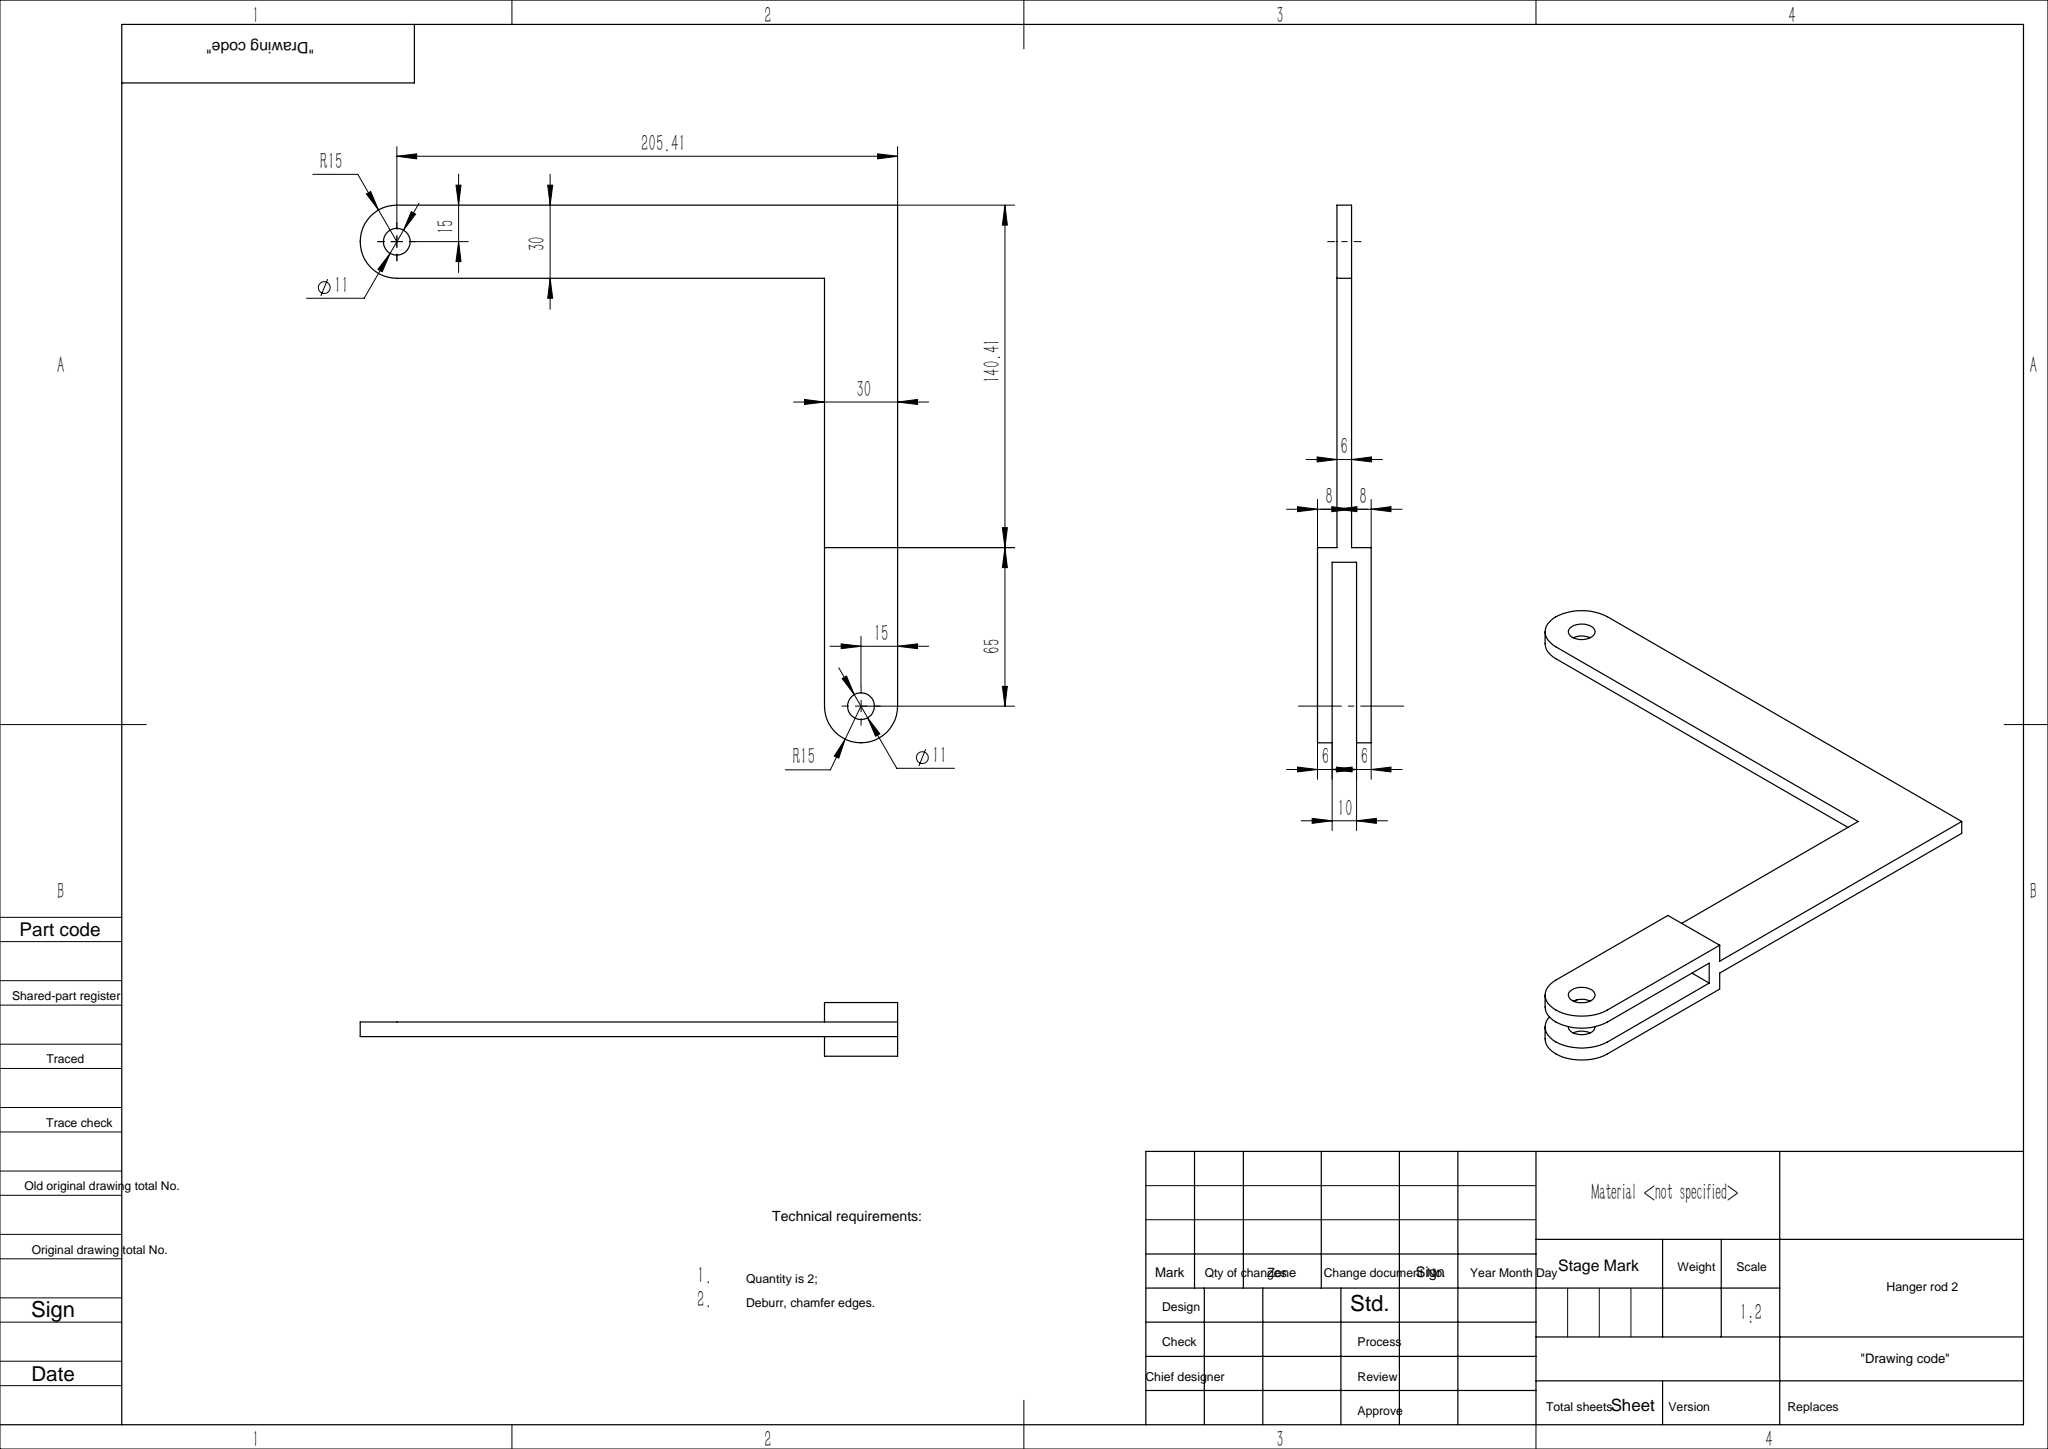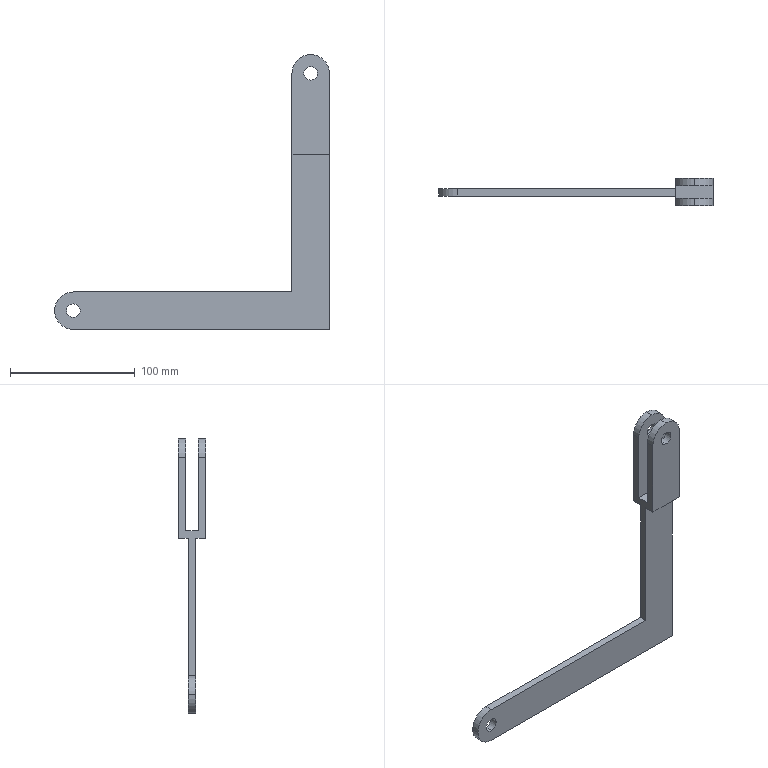Part | SolidWorks | features ICE 4, Fillet 2, Extrusion 1 | 1 solid | 25 faces | box 220.41 x 22 x 220.41 mm | volume 86699 mm3 | plane 13 | cylinder 12 | commonest cylinder face diameters 11 x6 30 x6
STEP:
#1=CARTESIAN_POINT('',(0.,-2.,-9.5));
#2=VERTEX_POINT('',#1);
#3=CARTESIAN_POINT('',(0.,-2.,-20.5));
#4=VERTEX_POINT('',#3);
#5=CARTESIAN_POINT('',(0.,-2.,-15.));
#6=DIRECTION('',(0.,-1.,0.));
#7=DIRECTION('',(0.,0.,-1.));
#8=AXIS2_PLACEMENT_3D('',#5,#6,#7);
#9=CIRCLE('',#8,5.5);
#10=EDGE_CURVE('',#2,#4,#9,.T.);
#11=ORIENTED_EDGE('',*,*,#10,.F.);
#12=CARTESIAN_POINT('',(0.,-8.,-9.5));
#13=VERTEX_POINT('',#12);
#14=CARTESIAN_POINT('',(0.,-2.,-9.5));
#15=DIRECTION('',(0.,-1.,0.));
#16=VECTOR('',#15,1000.);
#17=LINE('',#14,#16);
#18=EDGE_CURVE('',#2,#13,#17,.T.);
#19=ORIENTED_EDGE('',*,*,#18,.T.);
#20=CARTESIAN_POINT('',(0.,-8.,-20.5));
#21=VERTEX_POINT('',#20);
#22=CARTESIAN_POINT('',(0.,-8.,-15.));
#23=DIRECTION('',(0.,-1.,0.));
#24=DIRECTION('',(0.,0.,-1.));
#25=AXIS2_PLACEMENT_3D('',#22,#23,#24);
#26=CIRCLE('',#25,5.5);
#27=EDGE_CURVE('',#13,#21,#26,.T.);
#28=ORIENTED_EDGE('',*,*,#27,.T.);
#29=CARTESIAN_POINT('',(0.,-2.,-20.5));
#30=DIRECTION('',(0.,-1.,0.));
#31=VECTOR('',#30,1000.);
#32=LINE('',#29,#31);
#33=EDGE_CURVE('',#4,#21,#32,.T.);
#34=ORIENTED_EDGE('',*,*,#33,.F.);
#35=EDGE_LOOP('',(#11,#19,#28,#34));
#36=FACE_OUTER_BOUND('',#35,.T.);
#37=CARTESIAN_POINT('',(0.,-2.,-15.));
#38=DIRECTION('',(0.,-1.,0.));
#39=DIRECTION('',(0.,0.,-1.));
#40=AXIS2_PLACEMENT_3D('',#37,#38,#39);
#41=CYLINDRICAL_SURFACE('',#40,5.5);
#42=ADVANCED_FACE('',(#36),#41,.F.);
#43=CARTESIAN_POINT('',(0.,8.,-20.5));
#44=VERTEX_POINT('',#43);
#45=CARTESIAN_POINT('',(0.,8.,-9.5));
#46=VERTEX_POINT('',#45);
#47=CARTESIAN_POINT('',(0.,8.,-15.));
#48=DIRECTION('',(0.,1.,0.));
#49=DIRECTION('',(0.,0.,1.));
#50=AXIS2_PLACEMENT_3D('',#47,#48,#49);
#51=CIRCLE('',#50,5.5);
#52=EDGE_CURVE('',#44,#46,#51,.T.);
#53=ORIENTED_EDGE('',*,*,#52,.F.);
#54=CARTESIAN_POINT('',(0.,14.,-20.5));
#55=VERTEX_POINT('',#54);
#56=CARTESIAN_POINT('',(0.,8.,-20.5));
#57=DIRECTION('',(0.,1.,0.));
#58=VECTOR('',#57,1000.);
#59=LINE('',#56,#58);
#60=EDGE_CURVE('',#44,#55,#59,.T.);
#61=ORIENTED_EDGE('',*,*,#60,.T.);
#62=CARTESIAN_POINT('',(0.,14.,-9.5));
#63=VERTEX_POINT('',#62);
#64=CARTESIAN_POINT('',(0.,14.,-15.));
#65=DIRECTION('',(0.,1.,0.));
#66=DIRECTION('',(0.,0.,1.));
#67=AXIS2_PLACEMENT_3D('',#64,#65,#66);
#68=CIRCLE('',#67,5.5);
#69=EDGE_CURVE('',#55,#63,#68,.T.);
#70=ORIENTED_EDGE('',*,*,#69,.T.);
#71=CARTESIAN_POINT('',(0.,8.,-9.5));
#72=DIRECTION('',(0.,1.,0.));
#73=VECTOR('',#72,1000.);
#74=LINE('',#71,#73);
#75=EDGE_CURVE('',#46,#63,#74,.T.);
#76=ORIENTED_EDGE('',*,*,#75,.F.);
#77=EDGE_LOOP('',(#53,#61,#70,#76));
#78=FACE_OUTER_BOUND('',#77,.T.);
#79=CARTESIAN_POINT('',(0.,8.,-15.));
#80=DIRECTION('',(0.,1.,0.));
#81=DIRECTION('',(0.,0.,1.));
#82=AXIS2_PLACEMENT_3D('',#79,#80,#81);
#83=CYLINDRICAL_SURFACE('',#82,5.5);
#84=ADVANCED_FACE('',(#78),#83,.F.);
#85=CARTESIAN_POINT('',(-190.41,6.,-210.91));
#86=VERTEX_POINT('',#85);
#87=CARTESIAN_POINT('',(-190.41,6.,-199.91));
#88=VERTEX_POINT('',#87);
#89=CARTESIAN_POINT('',(-190.41,6.,-205.41));
#90=DIRECTION('',(0.,1.,0.));
#91=DIRECTION('',(0.,0.,1.));
#92=AXIS2_PLACEMENT_3D('',#89,#90,#91);
#93=CIRCLE('',#92,5.5);
#94=EDGE_CURVE('',#86,#88,#93,.T.);
#95=ORIENTED_EDGE('',*,*,#94,.T.);
#96=CARTESIAN_POINT('',(-190.41,0.,-199.91));
#97=VERTEX_POINT('',#96);
#98=CARTESIAN_POINT('',(-190.41,6.,-199.91));
#99=DIRECTION('',(0.,-1.,0.));
#100=VECTOR('',#99,1000.);
#101=LINE('',#98,#100);
#102=EDGE_CURVE('',#88,#97,#101,.T.);
#103=ORIENTED_EDGE('',*,*,#102,.T.);
#104=CARTESIAN_POINT('',(-190.41,0.,-210.91));
#105=VERTEX_POINT('',#104);
#106=CARTESIAN_POINT('',(-190.41,0.,-205.41));
#107=DIRECTION('',(0.,1.,0.));
#108=DIRECTION('',(0.,0.,1.));
#109=AXIS2_PLACEMENT_3D('',#106,#107,#108);
#110=CIRCLE('',#109,5.5);
#111=EDGE_CURVE('',#105,#97,#110,.T.);
#112=ORIENTED_EDGE('',*,*,#111,.F.);
#113=CARTESIAN_POINT('',(-190.41,6.,-210.91));
#114=DIRECTION('',(0.,-1.,0.));
#115=VECTOR('',#114,1000.);
#116=LINE('',#113,#115);
#117=EDGE_CURVE('',#86,#105,#116,.T.);
#118=ORIENTED_EDGE('',*,*,#117,.F.);
#119=EDGE_LOOP('',(#95,#103,#112,#118));
#120=FACE_OUTER_BOUND('',#119,.T.);
#121=CARTESIAN_POINT('',(-190.41,6.,-205.41));
#122=DIRECTION('',(0.,-1.,0.));
#123=DIRECTION('',(0.,0.,-1.));
#124=AXIS2_PLACEMENT_3D('',#121,#122,#123);
#125=CYLINDRICAL_SURFACE('',#124,5.5);
#126=ADVANCED_FACE('',(#120),#125,.F.);
#127=ORIENTED_EDGE('',*,*,#94,.F.);
#128=CARTESIAN_POINT('',(-190.41,6.,-205.41));
#129=DIRECTION('',(0.,1.,0.));
#130=DIRECTION('',(0.,0.,1.));
#131=AXIS2_PLACEMENT_3D('',#128,#129,#130);
#132=CIRCLE('',#131,5.5);
#133=EDGE_CURVE('',#88,#86,#132,.T.);
#134=ORIENTED_EDGE('',*,*,#133,.F.);
#135=EDGE_LOOP('',(#127,#134));
#136=FACE_BOUND('',#135,.T.);
#137=CARTESIAN_POINT('',(-15.,6.,-190.41));
#138=VERTEX_POINT('',#137);
#139=CARTESIAN_POINT('',(-15.,6.,-80.));
#140=VERTEX_POINT('',#139);
#141=CARTESIAN_POINT('',(-15.,6.,0.));
#142=DIRECTION('',(0.,0.,1.));
#143=VECTOR('',#142,1000.);
#144=LINE('',#141,#143);
#145=EDGE_CURVE('',#138,#140,#144,.T.);
#146=ORIENTED_EDGE('',*,*,#145,.T.);
#147=CARTESIAN_POINT('',(15.,6.,-80.));
#148=VERTEX_POINT('',#147);
#149=CARTESIAN_POINT('',(0.,6.,-80.));
#150=DIRECTION('',(1.,0.,0.));
#151=VECTOR('',#150,1000.);
#152=LINE('',#149,#151);
#153=EDGE_CURVE('',#140,#148,#152,.T.);
#154=ORIENTED_EDGE('',*,*,#153,.T.);
#155=CARTESIAN_POINT('',(15.,6.,-220.41));
#156=VERTEX_POINT('',#155);
#157=CARTESIAN_POINT('',(15.,6.,0.));
#158=DIRECTION('',(0.,0.,-1.));
#159=VECTOR('',#158,1000.);
#160=LINE('',#157,#159);
#161=EDGE_CURVE('',#148,#156,#160,.T.);
#162=ORIENTED_EDGE('',*,*,#161,.T.);
#163=CARTESIAN_POINT('',(-190.41,6.,-220.41));
#164=VERTEX_POINT('',#163);
#165=CARTESIAN_POINT('',(15.,6.,-220.41));
#166=DIRECTION('',(-1.,0.,0.));
#167=VECTOR('',#166,1000.);
#168=LINE('',#165,#167);
#169=EDGE_CURVE('',#156,#164,#168,.T.);
#170=ORIENTED_EDGE('',*,*,#169,.T.);
#171=CARTESIAN_POINT('',(-205.41,6.,-205.41));
#172=VERTEX_POINT('',#171);
#173=CARTESIAN_POINT('',(-190.41,6.,-205.41));
#174=DIRECTION('',(0.,1.,0.));
#175=DIRECTION('',(0.,0.,-1.));
#176=AXIS2_PLACEMENT_3D('',#173,#174,#175);
#177=CIRCLE('',#176,15.);
#178=EDGE_CURVE('',#164,#172,#177,.T.);
#179=ORIENTED_EDGE('',*,*,#178,.T.);
#180=CARTESIAN_POINT('',(-190.41,6.,-190.41));
#181=VERTEX_POINT('',#180);
#182=CARTESIAN_POINT('',(-190.41,6.,-205.41));
#183=DIRECTION('',(0.,1.,0.));
#184=DIRECTION('',(0.,0.,-1.));
#185=AXIS2_PLACEMENT_3D('',#182,#183,#184);
#186=CIRCLE('',#185,15.);
#187=EDGE_CURVE('',#172,#181,#186,.T.);
#188=ORIENTED_EDGE('',*,*,#187,.T.);
#189=CARTESIAN_POINT('',(-15.,6.,-190.41));
#190=DIRECTION('',(1.,0.,0.));
#191=VECTOR('',#190,1000.);
#192=LINE('',#189,#191);
#193=EDGE_CURVE('',#181,#138,#192,.T.);
#194=ORIENTED_EDGE('',*,*,#193,.T.);
#195=EDGE_LOOP('',(#146,#154,#162,#170,#179,#188,#194));
#196=FACE_OUTER_BOUND('',#195,.T.);
#197=CARTESIAN_POINT('',(0.,6.,0.));
#198=DIRECTION('',(0.,-1.,0.));
#199=DIRECTION('',(0.,0.,-1.));
#200=AXIS2_PLACEMENT_3D('',#197,#198,#199);
#201=PLANE('',#200);
#202=ADVANCED_FACE('',(#136,#196),#201,.F.);
#203=CARTESIAN_POINT('',(-15.,0.,-80.));
#204=VERTEX_POINT('',#203);
#205=CARTESIAN_POINT('',(15.,0.,-80.));
#206=VERTEX_POINT('',#205);
#207=CARTESIAN_POINT('',(0.,0.,-80.));
#208=DIRECTION('',(1.,0.,0.));
#209=VECTOR('',#208,1000.);
#210=LINE('',#207,#209);
#211=EDGE_CURVE('',#204,#206,#210,.T.);
#212=ORIENTED_EDGE('',*,*,#211,.F.);
#213=CARTESIAN_POINT('',(-15.,0.,-190.41));
#214=VERTEX_POINT('',#213);
#215=CARTESIAN_POINT('',(-15.,0.,0.));
#216=DIRECTION('',(0.,0.,1.));
#217=VECTOR('',#216,1000.);
#218=LINE('',#215,#217);
#219=EDGE_CURVE('',#214,#204,#218,.T.);
#220=ORIENTED_EDGE('',*,*,#219,.F.);
#221=CARTESIAN_POINT('',(-190.41,0.,-190.41));
#222=VERTEX_POINT('',#221);
#223=CARTESIAN_POINT('',(-15.,0.,-190.41));
#224=DIRECTION('',(1.,0.,0.));
#225=VECTOR('',#224,1000.);
#226=LINE('',#223,#225);
#227=EDGE_CURVE('',#222,#214,#226,.T.);
#228=ORIENTED_EDGE('',*,*,#227,.F.);
#229=CARTESIAN_POINT('',(-205.41,0.,-205.41));
#230=VERTEX_POINT('',#229);
#231=CARTESIAN_POINT('',(-190.41,0.,-205.41));
#232=DIRECTION('',(0.,-1.,0.));
#233=DIRECTION('',(0.,0.,-1.));
#234=AXIS2_PLACEMENT_3D('',#231,#232,#233);
#235=CIRCLE('',#234,15.);
#236=EDGE_CURVE('',#222,#230,#235,.T.);
#237=ORIENTED_EDGE('',*,*,#236,.T.);
#238=CARTESIAN_POINT('',(-190.41,0.,-220.41));
#239=VERTEX_POINT('',#238);
#240=CARTESIAN_POINT('',(-190.41,0.,-205.41));
#241=DIRECTION('',(0.,-1.,0.));
#242=DIRECTION('',(0.,0.,-1.));
#243=AXIS2_PLACEMENT_3D('',#240,#241,#242);
#244=CIRCLE('',#243,15.);
#245=EDGE_CURVE('',#230,#239,#244,.T.);
#246=ORIENTED_EDGE('',*,*,#245,.T.);
#247=CARTESIAN_POINT('',(15.,0.,-220.41));
#248=VERTEX_POINT('',#247);
#249=CARTESIAN_POINT('',(15.,0.,-220.41));
#250=DIRECTION('',(-1.,0.,0.));
#251=VECTOR('',#250,1000.);
#252=LINE('',#249,#251);
#253=EDGE_CURVE('',#248,#239,#252,.T.);
#254=ORIENTED_EDGE('',*,*,#253,.F.);
#255=CARTESIAN_POINT('',(15.,0.,0.));
#256=DIRECTION('',(0.,0.,-1.));
#257=VECTOR('',#256,1000.);
#258=LINE('',#255,#257);
#259=EDGE_CURVE('',#206,#248,#258,.T.);
#260=ORIENTED_EDGE('',*,*,#259,.F.);
#261=EDGE_LOOP('',(#212,#220,#228,#237,#246,#254,#260));
#262=FACE_OUTER_BOUND('',#261,.T.);
#263=ORIENTED_EDGE('',*,*,#111,.T.);
#264=CARTESIAN_POINT('',(-190.41,0.,-205.41));
#265=DIRECTION('',(0.,1.,0.));
#266=DIRECTION('',(0.,0.,1.));
#267=AXIS2_PLACEMENT_3D('',#264,#265,#266);
#268=CIRCLE('',#267,5.5);
#269=EDGE_CURVE('',#97,#105,#268,.T.);
#270=ORIENTED_EDGE('',*,*,#269,.T.);
#271=EDGE_LOOP('',(#263,#270));
#272=FACE_BOUND('',#271,.T.);
#273=CARTESIAN_POINT('',(0.,0.,0.));
#274=DIRECTION('',(0.,-1.,0.));
#275=DIRECTION('',(0.,0.,-1.));
#276=AXIS2_PLACEMENT_3D('',#273,#274,#275);
#277=PLANE('',#276);
#278=ADVANCED_FACE('',(#262,#272),#277,.T.);
#279=CARTESIAN_POINT('',(15.,14.,-15.));
#280=VERTEX_POINT('',#279);
#281=CARTESIAN_POINT('',(15.,14.,-80.));
#282=VERTEX_POINT('',#281);
#283=CARTESIAN_POINT('',(15.,14.,-80.));
#284=DIRECTION('',(0.,0.,-1.));
#285=VECTOR('',#284,1000.);
#286=LINE('',#283,#285);
#287=EDGE_CURVE('',#280,#282,#286,.T.);
#288=ORIENTED_EDGE('',*,*,#287,.F.);
#289=CARTESIAN_POINT('',(15.,8.,-15.));
#290=VERTEX_POINT('',#289);
#291=CARTESIAN_POINT('',(15.,8.,-15.));
#292=DIRECTION('',(0.,-1.,0.));
#293=VECTOR('',#292,1000.);
#294=LINE('',#291,#293);
#295=EDGE_CURVE('',#280,#290,#294,.T.);
#296=ORIENTED_EDGE('',*,*,#295,.T.);
#297=CARTESIAN_POINT('',(15.,8.,-74.));
#298=VERTEX_POINT('',#297);
#299=CARTESIAN_POINT('',(15.,8.,0.));
#300=DIRECTION('',(0.,0.,-1.));
#301=VECTOR('',#300,1000.);
#302=LINE('',#299,#301);
#303=EDGE_CURVE('',#290,#298,#302,.T.);
#304=ORIENTED_EDGE('',*,*,#303,.T.);
#305=CARTESIAN_POINT('',(15.,-2.,-74.));
#306=VERTEX_POINT('',#305);
#307=CARTESIAN_POINT('',(15.,-8.,-74.));
#308=DIRECTION('',(0.,1.,0.));
#309=VECTOR('',#308,1000.);
#310=LINE('',#307,#309);
#311=EDGE_CURVE('',#306,#298,#310,.T.);
#312=ORIENTED_EDGE('',*,*,#311,.F.);
#313=CARTESIAN_POINT('',(15.,-2.,-15.));
#314=VERTEX_POINT('',#313);
#315=CARTESIAN_POINT('',(15.,-2.,0.));
#316=DIRECTION('',(0.,0.,1.));
#317=VECTOR('',#316,1000.);
#318=LINE('',#315,#317);
#319=EDGE_CURVE('',#306,#314,#318,.T.);
#320=ORIENTED_EDGE('',*,*,#319,.T.);
#321=CARTESIAN_POINT('',(15.,-8.,-15.));
#322=VERTEX_POINT('',#321);
#323=CARTESIAN_POINT('',(15.,-8.,-15.));
#324=DIRECTION('',(0.,-1.,0.));
#325=VECTOR('',#324,1000.);
#326=LINE('',#323,#325);
#327=EDGE_CURVE('',#314,#322,#326,.T.);
#328=ORIENTED_EDGE('',*,*,#327,.T.);
#329=CARTESIAN_POINT('',(15.,-8.,-80.));
#330=VERTEX_POINT('',#329);
#331=CARTESIAN_POINT('',(15.,-8.,-80.));
#332=DIRECTION('',(0.,0.,-1.));
#333=VECTOR('',#332,1000.);
#334=LINE('',#331,#333);
#335=EDGE_CURVE('',#322,#330,#334,.T.);
#336=ORIENTED_EDGE('',*,*,#335,.T.);
#337=CARTESIAN_POINT('',(15.,-8.,-80.));
#338=DIRECTION('',(0.,1.,0.));
#339=VECTOR('',#338,1000.);
#340=LINE('',#337,#339);
#341=EDGE_CURVE('',#330,#206,#340,.T.);
#342=ORIENTED_EDGE('',*,*,#341,.T.);
#343=ORIENTED_EDGE('',*,*,#259,.T.);
#344=CARTESIAN_POINT('',(15.,6.,-220.41));
#345=DIRECTION('',(0.,-1.,0.));
#346=VECTOR('',#345,1000.);
#347=LINE('',#344,#346);
#348=EDGE_CURVE('',#156,#248,#347,.T.);
#349=ORIENTED_EDGE('',*,*,#348,.F.);
#350=ORIENTED_EDGE('',*,*,#161,.F.);
#351=CARTESIAN_POINT('',(15.,-8.,-80.));
#352=DIRECTION('',(0.,1.,0.));
#353=VECTOR('',#352,1000.);
#354=LINE('',#351,#353);
#355=EDGE_CURVE('',#148,#282,#354,.T.);
#356=ORIENTED_EDGE('',*,*,#355,.T.);
#357=EDGE_LOOP('',(#288,#296,#304,#312,#320,#328,#336,#342,#343,#349,#350,#356));
#358=FACE_OUTER_BOUND('',#357,.T.);
#359=CARTESIAN_POINT('',(15.,6.,0.));
#360=DIRECTION('',(-1.,0.,0.));
#361=DIRECTION('',(0.,0.,1.));
#362=AXIS2_PLACEMENT_3D('',#359,#360,#361);
#363=PLANE('',#362);
#364=ADVANCED_FACE('',(#358),#363,.F.);
#365=ORIENTED_EDGE('',*,*,#253,.T.);
#366=CARTESIAN_POINT('',(-190.41,6.,-220.41));
#367=DIRECTION('',(0.,1.,0.));
#368=VECTOR('',#367,1000.);
#369=LINE('',#366,#368);
#370=EDGE_CURVE('',#239,#164,#369,.T.);
#371=ORIENTED_EDGE('',*,*,#370,.T.);
#372=ORIENTED_EDGE('',*,*,#169,.F.);
#373=ORIENTED_EDGE('',*,*,#348,.T.);
#374=EDGE_LOOP('',(#365,#371,#372,#373));
#375=FACE_OUTER_BOUND('',#374,.T.);
#376=CARTESIAN_POINT('',(15.,6.,-220.41));
#377=DIRECTION('',(0.,0.,1.));
#378=DIRECTION('',(1.,0.,0.));
#379=AXIS2_PLACEMENT_3D('',#376,#377,#378);
#380=PLANE('',#379);
#381=ADVANCED_FACE('',(#375),#380,.F.);
#382=ORIENTED_EDGE('',*,*,#193,.F.);
#383=CARTESIAN_POINT('',(-190.41,6.,-190.41));
#384=DIRECTION('',(0.,-1.,0.));
#385=VECTOR('',#384,1000.);
#386=LINE('',#383,#385);
#387=EDGE_CURVE('',#181,#222,#386,.T.);
#388=ORIENTED_EDGE('',*,*,#387,.T.);
#389=ORIENTED_EDGE('',*,*,#227,.T.);
#390=CARTESIAN_POINT('',(-15.,6.,-190.41));
#391=DIRECTION('',(0.,-1.,0.));
#392=VECTOR('',#391,1000.);
#393=LINE('',#390,#392);
#394=EDGE_CURVE('',#138,#214,#393,.T.);
#395=ORIENTED_EDGE('',*,*,#394,.F.);
#396=EDGE_LOOP('',(#382,#388,#389,#395));
#397=FACE_OUTER_BOUND('',#396,.T.);
#398=CARTESIAN_POINT('',(-15.,6.,-190.41));
#399=DIRECTION('',(0.,0.,-1.));
#400=DIRECTION('',(-1.,0.,0.));
#401=AXIS2_PLACEMENT_3D('',#398,#399,#400);
#402=PLANE('',#401);
#403=ADVANCED_FACE('',(#397),#402,.F.);
#404=CARTESIAN_POINT('',(-15.,8.,-74.));
#405=VERTEX_POINT('',#404);
#406=CARTESIAN_POINT('',(-15.,8.,-15.));
#407=VERTEX_POINT('',#406);
#408=CARTESIAN_POINT('',(-15.,8.,-74.));
#409=DIRECTION('',(0.,0.,1.));
#410=VECTOR('',#409,1000.);
#411=LINE('',#408,#410);
#412=EDGE_CURVE('',#405,#407,#411,.T.);
#413=ORIENTED_EDGE('',*,*,#412,.T.);
#414=CARTESIAN_POINT('',(-15.,14.,-15.));
#415=VERTEX_POINT('',#414);
#416=CARTESIAN_POINT('',(-15.,14.,-15.));
#417=DIRECTION('',(0.,1.,0.));
#418=VECTOR('',#417,1000.);
#419=LINE('',#416,#418);
#420=EDGE_CURVE('',#407,#415,#419,.T.);
#421=ORIENTED_EDGE('',*,*,#420,.T.);
#422=CARTESIAN_POINT('',(-15.,14.,-80.));
#423=VERTEX_POINT('',#422);
#424=CARTESIAN_POINT('',(-15.,14.,-80.));
#425=DIRECTION('',(0.,0.,1.));
#426=VECTOR('',#425,1000.);
#427=LINE('',#424,#426);
#428=EDGE_CURVE('',#423,#415,#427,.T.);
#429=ORIENTED_EDGE('',*,*,#428,.F.);
#430=CARTESIAN_POINT('',(-15.,-8.,-80.));
#431=DIRECTION('',(0.,1.,0.));
#432=VECTOR('',#431,1000.);
#433=LINE('',#430,#432);
#434=EDGE_CURVE('',#140,#423,#433,.T.);
#435=ORIENTED_EDGE('',*,*,#434,.F.);
#436=ORIENTED_EDGE('',*,*,#145,.F.);
#437=ORIENTED_EDGE('',*,*,#394,.T.);
#438=ORIENTED_EDGE('',*,*,#219,.T.);
#439=CARTESIAN_POINT('',(-15.,-8.,-80.));
#440=VERTEX_POINT('',#439);
#441=CARTESIAN_POINT('',(-15.,-8.,-80.));
#442=DIRECTION('',(0.,1.,0.));
#443=VECTOR('',#442,1000.);
#444=LINE('',#441,#443);
#445=EDGE_CURVE('',#440,#204,#444,.T.);
#446=ORIENTED_EDGE('',*,*,#445,.F.);
#447=CARTESIAN_POINT('',(-15.,-8.,-15.));
#448=VERTEX_POINT('',#447);
#449=CARTESIAN_POINT('',(-15.,-8.,-80.));
#450=DIRECTION('',(0.,0.,1.));
#451=VECTOR('',#450,1000.);
#452=LINE('',#449,#451);
#453=EDGE_CURVE('',#440,#448,#452,.T.);
#454=ORIENTED_EDGE('',*,*,#453,.T.);
#455=CARTESIAN_POINT('',(-15.,-2.,-15.));
#456=VERTEX_POINT('',#455);
#457=CARTESIAN_POINT('',(-15.,-2.,-15.));
#458=DIRECTION('',(0.,1.,0.));
#459=VECTOR('',#458,1000.);
#460=LINE('',#457,#459);
#461=EDGE_CURVE('',#448,#456,#460,.T.);
#462=ORIENTED_EDGE('',*,*,#461,.T.);
#463=CARTESIAN_POINT('',(-15.,-2.,-74.));
#464=VERTEX_POINT('',#463);
#465=CARTESIAN_POINT('',(-15.,-2.,-74.));
#466=DIRECTION('',(0.,0.,-1.));
#467=VECTOR('',#466,1000.);
#468=LINE('',#465,#467);
#469=EDGE_CURVE('',#456,#464,#468,.T.);
#470=ORIENTED_EDGE('',*,*,#469,.T.);
#471=CARTESIAN_POINT('',(-15.,-8.,-74.));
#472=DIRECTION('',(0.,1.,0.));
#473=VECTOR('',#472,1000.);
#474=LINE('',#471,#473);
#475=EDGE_CURVE('',#464,#405,#474,.T.);
#476=ORIENTED_EDGE('',*,*,#475,.T.);
#477=EDGE_LOOP('',(#413,#421,#429,#435,#436,#437,#438,#446,#454,#462,#470,#476));
#478=FACE_OUTER_BOUND('',#477,.T.);
#479=CARTESIAN_POINT('',(-15.,6.,0.));
#480=DIRECTION('',(1.,0.,0.));
#481=DIRECTION('',(0.,0.,-1.));
#482=AXIS2_PLACEMENT_3D('',#479,#480,#481);
#483=PLANE('',#482);
#484=ADVANCED_FACE('',(#478),#483,.F.);
#485=ORIENTED_EDGE('',*,*,#102,.F.);
#486=ORIENTED_EDGE('',*,*,#133,.T.);
#487=ORIENTED_EDGE('',*,*,#117,.T.);
#488=ORIENTED_EDGE('',*,*,#269,.F.);
#489=EDGE_LOOP('',(#485,#486,#487,#488));
#490=FACE_OUTER_BOUND('',#489,.T.);
#491=CARTESIAN_POINT('',(-190.41,6.,-205.41));
#492=DIRECTION('',(0.,-1.,0.));
#493=DIRECTION('',(0.,0.,-1.));
#494=AXIS2_PLACEMENT_3D('',#491,#492,#493);
#495=CYLINDRICAL_SURFACE('',#494,5.5);
#496=ADVANCED_FACE('',(#490),#495,.F.);
#497=CARTESIAN_POINT('',(-205.41,6.,-205.41));
#498=DIRECTION('',(0.,-1.,0.));
#499=VECTOR('',#498,1000.);
#500=LINE('',#497,#499);
#501=EDGE_CURVE('',#172,#230,#500,.T.);
#502=ORIENTED_EDGE('',*,*,#501,.F.);
#503=ORIENTED_EDGE('',*,*,#178,.F.);
#504=ORIENTED_EDGE('',*,*,#370,.F.);
#505=ORIENTED_EDGE('',*,*,#245,.F.);
#506=EDGE_LOOP('',(#502,#503,#504,#505));
#507=FACE_OUTER_BOUND('',#506,.T.);
#508=CARTESIAN_POINT('',(-190.41,6.,-205.41));
#509=DIRECTION('',(0.,-1.,0.));
#510=DIRECTION('',(0.,0.,-1.));
#511=AXIS2_PLACEMENT_3D('',#508,#509,#510);
#512=CYLINDRICAL_SURFACE('',#511,15.);
#513=ADVANCED_FACE('',(#507),#512,.T.);
#514=ORIENTED_EDGE('',*,*,#187,.F.);
#515=ORIENTED_EDGE('',*,*,#501,.T.);
#516=ORIENTED_EDGE('',*,*,#236,.F.);
#517=ORIENTED_EDGE('',*,*,#387,.F.);
#518=EDGE_LOOP('',(#514,#515,#516,#517));
#519=FACE_OUTER_BOUND('',#518,.T.);
#520=CARTESIAN_POINT('',(-190.41,6.,-205.41));
#521=DIRECTION('',(0.,-1.,0.));
#522=DIRECTION('',(0.,0.,-1.));
#523=AXIS2_PLACEMENT_3D('',#520,#521,#522);
#524=CYLINDRICAL_SURFACE('',#523,15.);
#525=ADVANCED_FACE('',(#519),#524,.T.);
#526=ORIENTED_EDGE('',*,*,#335,.F.);
#527=CARTESIAN_POINT('',(0.,-8.,0.));
#528=VERTEX_POINT('',#527);
#529=CARTESIAN_POINT('',(0.,-8.,-15.));
#530=DIRECTION('',(0.,-1.,0.));
#531=DIRECTION('',(0.,0.,1.));
#532=AXIS2_PLACEMENT_3D('',#529,#530,#531);
#533=CIRCLE('',#532,15.);
#534=EDGE_CURVE('',#322,#528,#533,.T.);
#535=ORIENTED_EDGE('',*,*,#534,.T.);
#536=CARTESIAN_POINT('',(0.,-8.,-15.));
#537=DIRECTION('',(0.,-1.,0.));
#538=DIRECTION('',(0.,0.,1.));
#539=AXIS2_PLACEMENT_3D('',#536,#537,#538);
#540=CIRCLE('',#539,15.);
#541=EDGE_CURVE('',#528,#448,#540,.T.);
#542=ORIENTED_EDGE('',*,*,#541,.T.);
#543=ORIENTED_EDGE('',*,*,#453,.F.);
#544=CARTESIAN_POINT('',(-15.,-8.,-80.));
#545=DIRECTION('',(-1.,0.,0.));
#546=VECTOR('',#545,1000.);
#547=LINE('',#544,#546);
#548=EDGE_CURVE('',#330,#440,#547,.T.);
#549=ORIENTED_EDGE('',*,*,#548,.F.);
#550=EDGE_LOOP('',(#526,#535,#542,#543,#549));
#551=FACE_OUTER_BOUND('',#550,.T.);
#552=CARTESIAN_POINT('',(0.,-8.,-15.));
#553=DIRECTION('',(0.,-1.,0.));
#554=DIRECTION('',(0.,0.,-1.));
#555=AXIS2_PLACEMENT_3D('',#552,#553,#554);
#556=CIRCLE('',#555,5.5);
#557=EDGE_CURVE('',#21,#13,#556,.T.);
#558=ORIENTED_EDGE('',*,*,#557,.F.);
#559=ORIENTED_EDGE('',*,*,#27,.F.);
#560=EDGE_LOOP('',(#558,#559));
#561=FACE_BOUND('',#560,.T.);
#562=CARTESIAN_POINT('',(0.,-8.,0.));
#563=DIRECTION('',(0.,1.,0.));
#564=DIRECTION('',(0.,0.,1.));
#565=AXIS2_PLACEMENT_3D('',#562,#563,#564);
#566=PLANE('',#565);
#567=ADVANCED_FACE('',(#551,#561),#566,.F.);
#568=CARTESIAN_POINT('',(-15.,-2.,-74.));
#569=DIRECTION('',(1.,0.,0.));
#570=VECTOR('',#569,1000.);
#571=LINE('',#568,#570);
#572=EDGE_CURVE('',#464,#306,#571,.T.);
#573=ORIENTED_EDGE('',*,*,#572,.T.);
#574=ORIENTED_EDGE('',*,*,#311,.T.);
#575=CARTESIAN_POINT('',(15.,8.,-74.));
#576=DIRECTION('',(-1.,0.,0.));
#577=VECTOR('',#576,1000.);
#578=LINE('',#575,#577);
#579=EDGE_CURVE('',#298,#405,#578,.T.);
#580=ORIENTED_EDGE('',*,*,#579,.T.);
#581=ORIENTED_EDGE('',*,*,#475,.F.);
#582=EDGE_LOOP('',(#573,#574,#580,#581));
#583=FACE_OUTER_BOUND('',#582,.T.);
#584=CARTESIAN_POINT('',(-15.,-8.,-74.));
#585=DIRECTION('',(0.,0.,1.));
#586=DIRECTION('',(1.,0.,0.));
#587=AXIS2_PLACEMENT_3D('',#584,#585,#586);
#588=PLANE('',#587);
#589=ADVANCED_FACE('',(#583),#588,.T.);
#590=ORIENTED_EDGE('',*,*,#445,.T.);
#591=ORIENTED_EDGE('',*,*,#211,.T.);
#592=ORIENTED_EDGE('',*,*,#341,.F.);
#593=ORIENTED_EDGE('',*,*,#548,.T.);
#594=EDGE_LOOP('',(#590,#591,#592,#593));
#595=FACE_OUTER_BOUND('',#594,.T.);
#596=CARTESIAN_POINT('',(-15.,-8.,-80.));
#597=DIRECTION('',(0.,0.,-1.));
#598=DIRECTION('',(-1.,0.,0.));
#599=AXIS2_PLACEMENT_3D('',#596,#597,#598);
#600=PLANE('',#599);
#601=ADVANCED_FACE('',(#595),#600,.T.);
#602=ORIENTED_EDGE('',*,*,#153,.F.);
#603=ORIENTED_EDGE('',*,*,#434,.T.);
#604=CARTESIAN_POINT('',(-15.,14.,-80.));
#605=DIRECTION('',(-1.,0.,0.));
#606=VECTOR('',#605,1000.);
#607=LINE('',#604,#606);
#608=EDGE_CURVE('',#282,#423,#607,.T.);
#609=ORIENTED_EDGE('',*,*,#608,.F.);
#610=ORIENTED_EDGE('',*,*,#355,.F.);
#611=EDGE_LOOP('',(#602,#603,#609,#610));
#612=FACE_OUTER_BOUND('',#611,.T.);
#613=CARTESIAN_POINT('',(-15.,-8.,-80.));
#614=DIRECTION('',(0.,0.,-1.));
#615=DIRECTION('',(-1.,0.,0.));
#616=AXIS2_PLACEMENT_3D('',#613,#614,#615);
#617=PLANE('',#616);
#618=ADVANCED_FACE('',(#612),#617,.T.);
#619=CARTESIAN_POINT('',(0.,14.,0.));
#620=VERTEX_POINT('',#619);
#621=CARTESIAN_POINT('',(0.,14.,-15.));
#622=DIRECTION('',(0.,1.,0.));
#623=DIRECTION('',(0.,0.,1.));
#624=AXIS2_PLACEMENT_3D('',#621,#622,#623);
#625=CIRCLE('',#624,15.);
#626=EDGE_CURVE('',#415,#620,#625,.T.);
#627=ORIENTED_EDGE('',*,*,#626,.T.);
#628=CARTESIAN_POINT('',(0.,14.,-15.));
#629=DIRECTION('',(0.,1.,0.));
#630=DIRECTION('',(0.,0.,1.));
#631=AXIS2_PLACEMENT_3D('',#628,#629,#630);
#632=CIRCLE('',#631,15.);
#633=EDGE_CURVE('',#620,#280,#632,.T.);
#634=ORIENTED_EDGE('',*,*,#633,.T.);
#635=ORIENTED_EDGE('',*,*,#287,.T.);
#636=ORIENTED_EDGE('',*,*,#608,.T.);
#637=ORIENTED_EDGE('',*,*,#428,.T.);
#638=EDGE_LOOP('',(#627,#634,#635,#636,#637));
#639=FACE_OUTER_BOUND('',#638,.T.);
#640=CARTESIAN_POINT('',(0.,14.,-15.));
#641=DIRECTION('',(0.,1.,0.));
#642=DIRECTION('',(0.,0.,1.));
#643=AXIS2_PLACEMENT_3D('',#640,#641,#642);
#644=CIRCLE('',#643,5.5);
#645=EDGE_CURVE('',#63,#55,#644,.T.);
#646=ORIENTED_EDGE('',*,*,#645,.F.);
#647=ORIENTED_EDGE('',*,*,#69,.F.);
#648=EDGE_LOOP('',(#646,#647));
#649=FACE_BOUND('',#648,.T.);
#650=CARTESIAN_POINT('',(0.,14.,0.));
#651=DIRECTION('',(0.,1.,0.));
#652=DIRECTION('',(0.,0.,1.));
#653=AXIS2_PLACEMENT_3D('',#650,#651,#652);
#654=PLANE('',#653);
#655=ADVANCED_FACE('',(#639,#649),#654,.T.);
#656=CARTESIAN_POINT('',(0.,8.,-15.));
#657=DIRECTION('',(0.,1.,0.));
#658=DIRECTION('',(0.,0.,1.));
#659=AXIS2_PLACEMENT_3D('',#656,#657,#658);
#660=CIRCLE('',#659,5.5);
#661=EDGE_CURVE('',#46,#44,#660,.T.);
#662=ORIENTED_EDGE('',*,*,#661,.T.);
#663=ORIENTED_EDGE('',*,*,#52,.T.);
#664=EDGE_LOOP('',(#662,#663));
#665=FACE_BOUND('',#664,.T.);
#666=ORIENTED_EDGE('',*,*,#303,.F.);
#667=CARTESIAN_POINT('',(0.,8.,0.));
#668=VERTEX_POINT('',#667);
#669=CARTESIAN_POINT('',(0.,8.,-15.));
#670=DIRECTION('',(0.,-1.,0.));
#671=DIRECTION('',(0.,0.,1.));
#672=AXIS2_PLACEMENT_3D('',#669,#670,#671);
#673=CIRCLE('',#672,15.);
#674=EDGE_CURVE('',#290,#668,#673,.T.);
#675=ORIENTED_EDGE('',*,*,#674,.T.);
#676=CARTESIAN_POINT('',(0.,8.,-15.));
#677=DIRECTION('',(0.,-1.,0.));
#678=DIRECTION('',(0.,0.,1.));
#679=AXIS2_PLACEMENT_3D('',#676,#677,#678);
#680=CIRCLE('',#679,15.);
#681=EDGE_CURVE('',#668,#407,#680,.T.);
#682=ORIENTED_EDGE('',*,*,#681,.T.);
#683=ORIENTED_EDGE('',*,*,#412,.F.);
#684=ORIENTED_EDGE('',*,*,#579,.F.);
#685=EDGE_LOOP('',(#666,#675,#682,#683,#684));
#686=FACE_OUTER_BOUND('',#685,.T.);
#687=CARTESIAN_POINT('',(0.,8.,0.));
#688=DIRECTION('',(0.,1.,0.));
#689=DIRECTION('',(0.,0.,1.));
#690=AXIS2_PLACEMENT_3D('',#687,#688,#689);
#691=PLANE('',#690);
#692=ADVANCED_FACE('',(#665,#686),#691,.F.);
#693=ORIENTED_EDGE('',*,*,#60,.F.);
#694=ORIENTED_EDGE('',*,*,#661,.F.);
#695=ORIENTED_EDGE('',*,*,#75,.T.);
#696=ORIENTED_EDGE('',*,*,#645,.T.);
#697=EDGE_LOOP('',(#693,#694,#695,#696));
#698=FACE_OUTER_BOUND('',#697,.T.);
#699=CARTESIAN_POINT('',(0.,8.,-15.));
#700=DIRECTION('',(0.,1.,0.));
#701=DIRECTION('',(0.,0.,1.));
#702=AXIS2_PLACEMENT_3D('',#699,#700,#701);
#703=CYLINDRICAL_SURFACE('',#702,5.5);
#704=ADVANCED_FACE('',(#698),#703,.F.);
#705=CARTESIAN_POINT('',(0.,-2.,-15.));
#706=DIRECTION('',(0.,-1.,0.));
#707=DIRECTION('',(0.,0.,-1.));
#708=AXIS2_PLACEMENT_3D('',#705,#706,#707);
#709=CIRCLE('',#708,5.5);
#710=EDGE_CURVE('',#4,#2,#709,.T.);
#711=ORIENTED_EDGE('',*,*,#710,.T.);
#712=ORIENTED_EDGE('',*,*,#10,.T.);
#713=EDGE_LOOP('',(#711,#712));
#714=FACE_BOUND('',#713,.T.);
#715=CARTESIAN_POINT('',(0.,-2.,0.));
#716=VERTEX_POINT('',#715);
#717=CARTESIAN_POINT('',(0.,-2.,-15.));
#718=DIRECTION('',(0.,1.,0.));
#719=DIRECTION('',(0.,0.,1.));
#720=AXIS2_PLACEMENT_3D('',#717,#718,#719);
#721=CIRCLE('',#720,15.);
#722=EDGE_CURVE('',#456,#716,#721,.T.);
#723=ORIENTED_EDGE('',*,*,#722,.T.);
#724=CARTESIAN_POINT('',(0.,-2.,-15.));
#725=DIRECTION('',(0.,1.,0.));
#726=DIRECTION('',(0.,0.,1.));
#727=AXIS2_PLACEMENT_3D('',#724,#725,#726);
#728=CIRCLE('',#727,15.);
#729=EDGE_CURVE('',#716,#314,#728,.T.);
#730=ORIENTED_EDGE('',*,*,#729,.T.);
#731=ORIENTED_EDGE('',*,*,#319,.F.);
#732=ORIENTED_EDGE('',*,*,#572,.F.);
#733=ORIENTED_EDGE('',*,*,#469,.F.);
#734=EDGE_LOOP('',(#723,#730,#731,#732,#733));
#735=FACE_OUTER_BOUND('',#734,.T.);
#736=CARTESIAN_POINT('',(0.,-2.,0.));
#737=DIRECTION('',(0.,1.,0.));
#738=DIRECTION('',(0.,0.,1.));
#739=AXIS2_PLACEMENT_3D('',#736,#737,#738);
#740=PLANE('',#739);
#741=ADVANCED_FACE('',(#714,#735),#740,.T.);
#742=ORIENTED_EDGE('',*,*,#18,.F.);
#743=ORIENTED_EDGE('',*,*,#710,.F.);
#744=ORIENTED_EDGE('',*,*,#33,.T.);
#745=ORIENTED_EDGE('',*,*,#557,.T.);
#746=EDGE_LOOP('',(#742,#743,#744,#745));
#747=FACE_OUTER_BOUND('',#746,.T.);
#748=CARTESIAN_POINT('',(0.,-2.,-15.));
#749=DIRECTION('',(0.,-1.,0.));
#750=DIRECTION('',(0.,0.,-1.));
#751=AXIS2_PLACEMENT_3D('',#748,#749,#750);
#752=CYLINDRICAL_SURFACE('',#751,5.5);
#753=ADVANCED_FACE('',(#747),#752,.F.);
#754=ORIENTED_EDGE('',*,*,#420,.F.);
#755=ORIENTED_EDGE('',*,*,#681,.F.);
#756=CARTESIAN_POINT('',(0.,8.,0.));
#757=DIRECTION('',(0.,-1.,0.));
#758=VECTOR('',#757,1000.);
#759=LINE('',#756,#758);
#760=EDGE_CURVE('',#620,#668,#759,.T.);
#761=ORIENTED_EDGE('',*,*,#760,.F.);
#762=ORIENTED_EDGE('',*,*,#626,.F.);
#763=EDGE_LOOP('',(#754,#755,#761,#762));
#764=FACE_OUTER_BOUND('',#763,.T.);
#765=CARTESIAN_POINT('',(0.,6.,-15.));
#766=DIRECTION('',(0.,-1.,0.));
#767=DIRECTION('',(0.,0.,-1.));
#768=AXIS2_PLACEMENT_3D('',#765,#766,#767);
#769=CYLINDRICAL_SURFACE('',#768,15.);
#770=ADVANCED_FACE('',(#764),#769,.T.);
#771=ORIENTED_EDGE('',*,*,#674,.F.);
#772=ORIENTED_EDGE('',*,*,#295,.F.);
#773=ORIENTED_EDGE('',*,*,#633,.F.);
#774=ORIENTED_EDGE('',*,*,#760,.T.);
#775=EDGE_LOOP('',(#771,#772,#773,#774));
#776=FACE_OUTER_BOUND('',#775,.T.);
#777=CARTESIAN_POINT('',(0.,8.,-15.));
#778=DIRECTION('',(0.,-1.,0.));
#779=DIRECTION('',(0.,0.,-1.));
#780=AXIS2_PLACEMENT_3D('',#777,#778,#779);
#781=CYLINDRICAL_SURFACE('',#780,15.);
#782=ADVANCED_FACE('',(#776),#781,.T.);
#783=CARTESIAN_POINT('',(0.,-8.,0.));
#784=DIRECTION('',(0.,-1.,0.));
#785=VECTOR('',#784,1000.);
#786=LINE('',#783,#785);
#787=EDGE_CURVE('',#716,#528,#786,.T.);
#788=ORIENTED_EDGE('',*,*,#787,.F.);
#789=ORIENTED_EDGE('',*,*,#722,.F.);
#790=ORIENTED_EDGE('',*,*,#461,.F.);
#791=ORIENTED_EDGE('',*,*,#541,.F.);
#792=EDGE_LOOP('',(#788,#789,#790,#791));
#793=FACE_OUTER_BOUND('',#792,.T.);
#794=CARTESIAN_POINT('',(0.,-2.,-15.));
#795=DIRECTION('',(0.,1.,0.));
#796=DIRECTION('',(0.,0.,1.));
#797=AXIS2_PLACEMENT_3D('',#794,#795,#796);
#798=CYLINDRICAL_SURFACE('',#797,15.);
#799=ADVANCED_FACE('',(#793),#798,.T.);
#800=ORIENTED_EDGE('',*,*,#729,.F.);
#801=ORIENTED_EDGE('',*,*,#787,.T.);
#802=ORIENTED_EDGE('',*,*,#534,.F.);
#803=ORIENTED_EDGE('',*,*,#327,.F.);
#804=EDGE_LOOP('',(#800,#801,#802,#803));
#805=FACE_OUTER_BOUND('',#804,.T.);
#806=CARTESIAN_POINT('',(0.,6.,-15.));
#807=DIRECTION('',(0.,1.,0.));
#808=DIRECTION('',(0.,0.,1.));
#809=AXIS2_PLACEMENT_3D('',#806,#807,#808);
#810=CYLINDRICAL_SURFACE('',#809,15.);
#811=ADVANCED_FACE('',(#805),#810,.T.);
#812=CLOSED_SHELL('',(#42,#84,#126,#202,#278,#364,#381,#403,#484,#496,#513,#525,#567,#589,#601,#618,#655,#692,#704,#741,#753,#770,#782,#799,#811));
#813=MANIFOLD_SOLID_BREP('',#812);
#814=CARTESIAN_POINT('',(0.,0.,0.));
#815=DIRECTION('',(0.,0.,1.));
#816=DIRECTION('',(1.,0.,0.));
#817=AXIS2_PLACEMENT_3D('',#814,#815,#816);
#818=(LENGTH_UNIT()NAMED_UNIT(*)SI_UNIT(.MILLI.,.METRE.));
#819=UNCERTAINTY_MEASURE_WITH_UNIT(LENGTH_MEASURE(0.00001),#818,'','');
#820=(NAMED_UNIT(*)PLANE_ANGLE_UNIT()SI_UNIT($,.RADIAN.));
#821=(NAMED_UNIT(*)SI_UNIT($,.STERADIAN.)SOLID_ANGLE_UNIT());
#822=(GEOMETRIC_REPRESENTATION_CONTEXT(3)GLOBAL_UNCERTAINTY_ASSIGNED_CONTEXT((#819))GLOBAL_UNIT_ASSIGNED_CONTEXT((#818,#820,#821))REPRESENTATION_CONTEXT('',''));
#823=ADVANCED_BREP_SHAPE_REPRESENTATION('',(#813,#817),#822);